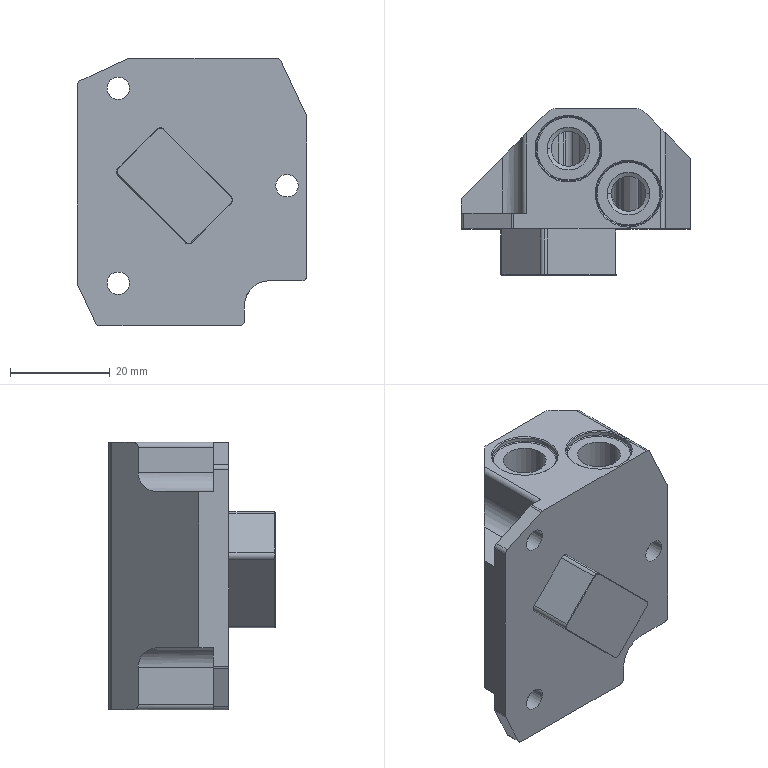NC program | NX | posted with a generic post | part box 46 x 33.25 x 53.5 mm
Whole program, first 1397 of 1693 lines:
N10 G17 G21 G94 G90
(PLANAR_MILL_7 , TOOL : D5-15-D6-50-3T-ROUGH)
N12 T03 M6
N14 G54
N16 G17 G0 G90 X1.887 Y-14.189 B0. C0. S4500 M3
N18 G43 Z20. H3
N20 Z1.
N22 G94 G1 X1.167 Y-14.167 Z0.975 F300.
N24 X0.474 Y-14.445 Z0.949
N26 X-0.055 Y-14.974 Z0.923
N28 X-0.333 Y-15.667 Z0.896
N30 Y-16.333 Z0.873
N32 X-0.055 Y-17.026 Z0.847
N34 X0.474 Y-17.555 Z0.821
N36 X1.167 Y-17.833 Z0.795
N38 X1.833 Z0.772
N40 X2.526 Y-17.555 Z0.746
N42 X3.055 Y-17.026 Z0.719
N44 X3.333 Y-16.333 Z0.693
N46 Y-15.667 Z0.67
N48 X3.055 Y-14.974 Z0.644
N50 X2.526 Y-14.445 Z0.618
N52 X1.833 Y-14.167 Z0.592
N54 X1.167 Z0.569
N56 X0.474 Y-14.445 Z0.542
N58 X-0.055 Y-14.974 Z0.516
N60 X-0.333 Y-15.667 Z0.49
N62 Y-16.333 Z0.467
N64 X-0.055 Y-17.026 Z0.441
N66 X0.474 Y-17.555 Z0.415
N68 X1.167 Y-17.833 Z0.389
N70 X1.833 Z0.366
N72 X2.526 Y-17.555 Z0.339
N74 X3.055 Y-17.026 Z0.313
N76 X3.333 Y-16.333 Z0.287
N78 Y-15.667 Z0.264
N80 X3.055 Y-14.974 Z0.238
N82 X2.526 Y-14.445 Z0.212
N84 X1.833 Y-14.167 Z0.186
N86 X1.167 Z0.162
N88 X0.474 Y-14.445 Z0.136
N90 X-0.055 Y-14.974 Z0.11
N92 X-0.333 Y-15.667 Z0.084
N94 Y-16.333 Z0.061
N96 X-0.055 Y-17.026 Z0.035
N98 X0.474 Y-17.555 Z0.009
N100 X1.167 Y-17.833 Z-0.017
N102 X1.833 Z-0.041
N104 X2.526 Y-17.555 Z-0.067
N106 X3.055 Y-17.026 Z-0.093
N108 X3.333 Y-16.333 Z-0.119
N110 Y-15.667 Z-0.142
N112 X3.055 Y-14.974 Z-0.168
N114 X2.526 Y-14.445 Z-0.194
N116 X1.833 Y-14.167 Z-0.22
N118 X1.167 Z-0.244
N120 X0.474 Y-14.445 Z-0.27
N122 X-0.055 Y-14.974 Z-0.296
N124 X-0.333 Y-15.667 Z-0.322
N126 Y-16.333 Z-0.345
N128 X-0.055 Y-17.026 Z-0.371
N130 X0.474 Y-17.555 Z-0.397
N132 X1.167 Y-17.833 Z-0.423
N134 X1.833 Z-0.447
N136 X2.526 Y-17.555 Z-0.473
N138 X3.055 Y-17.026 Z-0.499
N140 X3.333 Y-16.333 Z-0.525
N142 Y-15.667 Z-0.548
N144 X3.055 Y-14.974 Z-0.574
N146 X2.526 Y-14.445 Z-0.6
N148 X1.833 Y-14.167 Z-0.627
N150 X1.167 Z-0.65
N152 X0.474 Y-14.445 Z-0.676
N154 X-0.055 Y-14.974 Z-0.702
N156 X-0.333 Y-15.667 Z-0.728
N158 Y-16.333 Z-0.751
N160 X-0.055 Y-17.026 Z-0.777
N162 X0.474 Y-17.555 Z-0.804
N164 X1.167 Y-17.833 Z-0.83
N166 X1.833 Z-0.853
N168 X2.526 Y-17.555 Z-0.879
N170 X3.055 Y-17.026 Z-0.905
N172 X3.333 Y-16.333 Z-0.931
N174 Y-15.667 Z-0.954
N176 X3.055 Y-14.974 Z-0.98
N178 X2.526 Y-14.445 Z-1.007
N180 X1.833 Y-14.167 Z-1.033
N182 X1.167 Z-1.056
N184 X0.474 Y-14.445 Z-1.082
N186 X-0.055 Y-14.974 Z-1.108
N188 X-0.333 Y-15.667 Z-1.134
N190 Y-16.333 Z-1.157
N192 X-0.055 Y-17.026 Z-1.184
N194 X0.474 Y-17.555 Z-1.21
N196 X1.167 Y-17.833 Z-1.236
N198 X1.833 Z-1.259
N200 X2.526 Y-17.555 Z-1.285
N202 X3.055 Y-17.026 Z-1.311
N204 X3.333 Y-16.333 Z-1.337
N206 Y-15.667 Z-1.361
N208 X3.055 Y-14.974 Z-1.387
N210 X2.526 Y-14.445 Z-1.413
N212 X1.833 Y-14.167 Z-1.439
N214 X1.167 Z-1.462
N216 X0.474 Y-14.445 Z-1.488
N218 X-0.055 Y-14.974 Z-1.514
N220 X-0.333 Y-15.667 Z-1.54
N222 Y-16.333 Z-1.564
N224 X-0.055 Y-17.026 Z-1.59
N226 X0.474 Y-17.555 Z-1.616
N228 X1.167 Y-17.833 Z-1.642
N230 X1.833 Z-1.665
N232 X2.526 Y-17.555 Z-1.691
N234 X3.055 Y-17.026 Z-1.717
N236 X3.333 Y-16.333 Z-1.743
N238 Y-15.667 Z-1.767
N240 X3.055 Y-14.974 Z-1.793
N242 X2.526 Y-14.445 Z-1.819
N244 X1.833 Y-14.167 Z-1.845
N246 X1.167 Z-1.868
N248 X0.474 Y-14.445 Z-1.894
N250 X-0.055 Y-14.974 Z-1.92
N252 X-0.333 Y-15.667 Z-1.946
N254 Y-16.333 Z-1.97
N256 X-0.055 Y-17.026 Z-1.996
N258 X0.474 Y-17.555 Z-2.022
N260 X1.167 Y-17.833 Z-2.048
N262 X1.833 Z-2.071
N264 X2.526 Y-17.555 Z-2.097
N266 X3.055 Y-17.026 Z-2.123
N268 X3.333 Y-16.333 Z-2.15
N270 Y-15.667 Z-2.173
N272 X3.055 Y-14.974 Z-2.199
N274 X2.526 Y-14.445 Z-2.225
N276 X1.833 Y-14.167 Z-2.251
N278 X1.167 Z-2.274
N280 X0.474 Y-14.445 Z-2.3
N282 X-0.055 Y-14.974 Z-2.326
N284 X-0.333 Y-15.667 Z-2.353
N286 Y-16.333 Z-2.376
N288 X-0.055 Y-17.026 Z-2.402
N290 X0.474 Y-17.555 Z-2.428
N292 X1.167 Y-17.833 Z-2.454
N294 X1.833 Z-2.477
N296 X2.526 Y-17.555 Z-2.503
N298 X3.055 Y-17.026 Z-2.53
N300 X3.333 Y-16.333 Z-2.556
N302 Y-15.667 Z-2.579
N304 X3.055 Y-14.974 Z-2.605
N306 X2.526 Y-14.445 Z-2.631
N308 X1.833 Y-14.167 Z-2.657
N310 X1.167 Z-2.68
N312 X0.474 Y-14.445 Z-2.707
N314 X-0.055 Y-14.974 Z-2.733
N316 X-0.333 Y-15.667 Z-2.759
N318 Y-16.333 Z-2.782
N320 X-0.055 Y-17.026 Z-2.808
N322 X0.474 Y-17.555 Z-2.834
N324 X1.167 Y-17.833 Z-2.86
N326 X1.833 Z-2.884
N328 X2.526 Y-17.555 Z-2.91
N330 X3.055 Y-17.026 Z-2.936
N332 X3.333 Y-16.333 Z-2.962
N334 Y-15.667 Z-2.985
N336 X3.055 Y-14.974 Z-3.011
N338 X2.526 Y-14.445 Z-3.037
N340 X1.833 Y-14.167 Z-3.063
N342 X1.167 Z-3.087
N344 X0.474 Y-14.445 Z-3.113
N346 X-0.055 Y-14.974 Z-3.139
N348 X-0.333 Y-15.667 Z-3.165
N350 Y-16.333 Z-3.188
N352 X-0.055 Y-17.026 Z-3.214
N354 X0.474 Y-17.555 Z-3.24
N356 X1.167 Y-17.833 Z-3.266
N358 X1.833 Z-3.29
N360 X2.526 Y-17.555 Z-3.316
N362 X3.055 Y-17.026 Z-3.342
N364 X3.333 Y-16.333 Z-3.368
N366 Y-15.667 Z-3.391
N368 X3.055 Y-14.974 Z-3.417
N370 X2.526 Y-14.445 Z-3.443
N372 X1.833 Y-14.167 Z-3.469
N374 X1.167 Z-3.493
N376 X0.474 Y-14.445 Z-3.519
N378 X-0.055 Y-14.974 Z-3.545
N380 X-0.333 Y-15.667 Z-3.571
N382 Y-16.333 Z-3.594
N384 X-0.055 Y-17.026 Z-3.62
N386 X0.474 Y-17.555 Z-3.646
N388 X1.167 Y-17.833 Z-3.672
N390 X1.833 Z-3.696
N392 X2.526 Y-17.555 Z-3.722
N394 X3.055 Y-17.026 Z-3.748
N396 X3.333 Y-16.333 Z-3.774
N398 Y-15.667 Z-3.797
N400 X3.055 Y-14.974 Z-3.823
N402 X2.526 Y-14.445 Z-3.849
N404 X1.833 Y-14.167 Z-3.876
N406 X1.167 Z-3.899
N408 X0.474 Y-14.445 Z-3.925
N410 X-0.055 Y-14.974 Z-3.951
N412 X-0.333 Y-15.667 Z-3.977
N414 Y-16.333 Z-4.
N416 X-0.055 Y-17.026 Z-4.026
N418 X0.474 Y-17.555 Z-4.053
N420 X1.167 Y-17.833 Z-4.079
N422 X1.833 Z-4.102
N424 X2.526 Y-17.555 Z-4.128
N426 X3.055 Y-17.026 Z-4.154
N428 X3.333 Y-16.333 Z-4.18
N430 Y-15.667 Z-4.203
N432 X3.055 Y-14.974 Z-4.23
N434 X2.526 Y-14.445 Z-4.256
N436 X1.833 Y-14.167 Z-4.282
N438 X1.167 Z-4.305
N440 X0.474 Y-14.445 Z-4.331
N442 X-0.055 Y-14.974 Z-4.357
N444 X-0.333 Y-15.667 Z-4.383
N446 Y-16.333 Z-4.406
N448 X-0.055 Y-17.026 Z-4.433
N450 X0.474 Y-17.555 Z-4.459
N452 X1.167 Y-17.833 Z-4.485
N454 X1.833 Z-4.508
N456 X2.526 Y-17.555 Z-4.534
N458 X3.055 Y-17.026 Z-4.56
N460 X3.333 Y-16.333 Z-4.586
N462 Y-15.667 Z-4.61
N464 X3.055 Y-14.974 Z-4.636
N466 X2.526 Y-14.445 Z-4.662
N468 X1.833 Y-14.167 Z-4.688
N470 X1.167 Z-4.711
N472 X0.474 Y-14.445 Z-4.737
N474 X-0.055 Y-14.974 Z-4.763
N476 X-0.333 Y-15.667 Z-4.789
N478 Y-16.333 Z-4.813
N480 X-0.055 Y-17.026 Z-4.839
N482 X0.474 Y-17.555 Z-4.865
N484 X1.167 Y-17.833 Z-4.891
N486 X1.833 Z-4.914
N488 X2.526 Y-17.555 Z-4.94
N490 X3.055 Y-17.026 Z-4.966
N492 X3.333 Y-16.333 Z-4.992
N494 Y-15.667 Z-5.016
N496 X3.055 Y-14.974 Z-5.042
N498 X2.526 Y-14.445 Z-5.068
N500 X1.833 Y-14.167 Z-5.094
N502 X1.167 Z-5.117
N504 X0.474 Y-14.445 Z-5.143
N506 X-0.055 Y-14.974 Z-5.169
N508 X-0.333 Y-15.667 Z-5.195
N510 Y-16.333 Z-5.219
N512 X-0.055 Y-17.026 Z-5.245
N514 X0.474 Y-17.555 Z-5.271
N516 X1.167 Y-17.833 Z-5.297
N518 X1.833 Z-5.32
N520 X2.526 Y-17.555 Z-5.346
N522 X3.055 Y-17.026 Z-5.372
N524 X3.333 Y-16.333 Z-5.399
N526 Y-15.667 Z-5.422
N528 X3.055 Y-14.974 Z-5.448
N530 X2.526 Y-14.445 Z-5.474
N532 X1.833 Y-14.167 Z-5.5
N534 X1.167 Z-5.523
N536 X0.474 Y-14.445 Z-5.549
N538 X-0.055 Y-14.974 Z-5.576
N540 X-0.333 Y-15.667 Z-5.602
N542 Y-16.333 Z-5.625
N544 X-0.055 Y-17.026 Z-5.651
N546 X0.474 Y-17.555 Z-5.677
N548 X1.167 Y-17.833 Z-5.703
N550 X1.833 Z-5.726
N552 X2.526 Y-17.555 Z-5.752
N554 X3.055 Y-17.026 Z-5.779
N556 X3.333 Y-16.333 Z-5.805
N558 Y-15.667 Z-5.828
N560 X3.055 Y-14.974 Z-5.854
N562 X2.526 Y-14.445 Z-5.88
N564 X1.833 Y-14.167 Z-5.906
N566 X1.167 Z-5.929
N568 X0.474 Y-14.445 Z-5.956
N570 X-0.055 Y-14.974 Z-5.982
N572 X-0.333 Y-15.667 Z-6.008
N574 Y-16.333 Z-6.031
N576 X-0.055 Y-17.026 Z-6.057
N578 X0.474 Y-17.555 Z-6.083
N580 X1.167 Y-17.833 Z-6.109
N582 X1.833 Z-6.133
N584 X2.526 Y-17.555 Z-6.159
N586 X3.055 Y-17.026 Z-6.185
N588 X3.333 Y-16.333 Z-6.211
N590 Y-15.667 Z-6.234
N592 X3.055 Y-14.974 Z-6.26
N594 X2.526 Y-14.445 Z-6.286
N596 X1.833 Y-14.167 Z-6.312
N598 X1.167 Z-6.336
N600 X0.474 Y-14.445 Z-6.362
N602 X-0.055 Y-14.974 Z-6.388
N604 X-0.333 Y-15.667 Z-6.414
N606 Y-16.333 Z-6.437
N608 X-0.055 Y-17.026 Z-6.463
N610 X0.474 Y-17.555 Z-6.489
N612 X1.167 Y-17.833 Z-6.515
N614 X1.833 Z-6.539
N616 X2.526 Y-17.555 Z-6.565
N618 X3.055 Y-17.026 Z-6.591
N620 X3.333 Y-16.333 Z-6.617
N622 Y-15.667 Z-6.64
N624 X3.055 Y-14.974 Z-6.666
N626 X2.526 Y-14.445 Z-6.692
N628 X1.833 Y-14.167 Z-6.718
N630 X1.167 Z-6.742
N632 X0.474 Y-14.445 Z-6.768
N634 X-0.055 Y-14.974 Z-6.794
N636 X-0.333 Y-15.667 Z-6.82
N638 Y-16.333 Z-6.843
N640 X-0.055 Y-17.026 Z-6.869
N642 X0.474 Y-17.555 Z-6.895
N644 X1.167 Y-17.833 Z-6.922
N646 X1.833 Z-6.945
N648 X2.526 Y-17.555 Z-6.971
N650 X3.055 Y-17.026 Z-6.997
N652 X3.333 Y-16.333 Z-7.023
N654 Y-15.667 Z-7.046
N656 X3.055 Y-14.974 Z-7.072
N658 X2.526 Y-14.445 Z-7.098
N660 X1.833 Y-14.167 Z-7.125
N662 X1.167 Z-7.148
N664 X0.474 Y-14.445 Z-7.174
N666 X-0.055 Y-14.974 Z-7.2
N668 X-0.333 Y-15.667 Z-7.226
N670 Y-16.333 Z-7.249
N672 X-0.055 Y-17.026 Z-7.275
N674 X0.474 Y-17.555 Z-7.302
N676 X1.167 Y-17.833 Z-7.328
N678 X1.833 Z-7.351
N680 X2.526 Y-17.555 Z-7.377
N682 X3.055 Y-17.026 Z-7.403
N684 X3.333 Y-16.333 Z-7.429
N686 Y-15.667 Z-7.452
N688 X3.055 Y-14.974 Z-7.479
N690 X2.526 Y-14.445 Z-7.505
N692 X1.833 Y-14.167 Z-7.531
N694 X1.167 Z-7.554
N696 X0.474 Y-14.445 Z-7.58
N698 X-0.055 Y-14.974 Z-7.606
N700 X-0.333 Y-15.667 Z-7.632
N702 Y-16.333 Z-7.656
N704 X-0.055 Y-17.026 Z-7.682
N706 X0.474 Y-17.555 Z-7.708
N708 X1.167 Y-17.833 Z-7.734
N710 X1.833 Z-7.757
N712 X2.526 Y-17.555 Z-7.783
N714 X3.055 Y-17.026 Z-7.809
N716 X3.333 Y-16.333 Z-7.835
N718 Y-15.667 Z-7.859
N720 X3.055 Y-14.974 Z-7.885
N722 X2.526 Y-14.445 Z-7.911
N724 X1.833 Y-14.167 Z-7.937
N726 X1.167 Z-7.96
N728 X0.474 Y-14.445 Z-7.986
N730 X-0.055 Y-14.974 Z-8.012
N732 X-0.333 Y-15.667 Z-8.038
N734 Y-16. Z-8.05
N736 G3 X1.5 Y-17.833 R1.833
N738 X-0.333 Y-16. R-1.833
N740 G1 Z-7.05
N742 G0 Z20.
N744 X-10.113 Y-5.189
N746 Z1.
N748 G1 X-10.833 Y-5.167 Z0.975
N750 X-11.526 Y-5.445 Z0.949
N752 X-12.055 Y-5.974 Z0.923
N754 X-12.333 Y-6.667 Z0.896
N756 Y-7.333 Z0.873
N758 X-12.055 Y-8.026 Z0.847
N760 X-11.526 Y-8.555 Z0.821
N762 X-10.833 Y-8.833 Z0.795
N764 X-10.167 Z0.772
N766 X-9.474 Y-8.555 Z0.746
N768 X-8.945 Y-8.026 Z0.719
N770 X-8.667 Y-7.333 Z0.693
N772 Y-6.667 Z0.67
N774 X-8.945 Y-5.974 Z0.644
N776 X-9.474 Y-5.445 Z0.618
N778 X-10.167 Y-5.167 Z0.592
N780 X-10.833 Z0.569
N782 X-11.526 Y-5.445 Z0.542
N784 X-12.055 Y-5.974 Z0.516
N786 X-12.333 Y-6.667 Z0.49
N788 Y-7.333 Z0.467
N790 X-12.055 Y-8.026 Z0.441
N792 X-11.526 Y-8.555 Z0.415
N794 X-10.833 Y-8.833 Z0.389
N796 X-10.167 Z0.366
N798 X-9.474 Y-8.555 Z0.339
N800 X-8.945 Y-8.026 Z0.313
N802 X-8.667 Y-7.333 Z0.287
N804 Y-6.667 Z0.264
N806 X-8.945 Y-5.974 Z0.238
N808 X-9.474 Y-5.445 Z0.212
N810 X-10.167 Y-5.167 Z0.186
N812 X-10.833 Z0.162
N814 X-11.526 Y-5.445 Z0.136
N816 X-12.055 Y-5.974 Z0.11
N818 X-12.333 Y-6.667 Z0.084
N820 Y-7.333 Z0.061
N822 X-12.055 Y-8.026 Z0.035
N824 X-11.526 Y-8.555 Z0.009
N826 X-10.833 Y-8.833 Z-0.017
N828 X-10.167 Z-0.041
N830 X-9.474 Y-8.555 Z-0.067
N832 X-8.945 Y-8.026 Z-0.093
N834 X-8.667 Y-7.333 Z-0.119
N836 Y-6.667 Z-0.142
N838 X-8.945 Y-5.974 Z-0.168
N840 X-9.474 Y-5.445 Z-0.194
N842 X-10.167 Y-5.167 Z-0.22
N844 X-10.833 Z-0.244
N846 X-11.526 Y-5.445 Z-0.27
N848 X-12.055 Y-5.974 Z-0.296
N850 X-12.333 Y-6.667 Z-0.322
N852 Y-7.333 Z-0.345
N854 X-12.055 Y-8.026 Z-0.371
N856 X-11.526 Y-8.555 Z-0.397
N858 X-10.833 Y-8.833 Z-0.423
N860 X-10.167 Z-0.447
N862 X-9.474 Y-8.555 Z-0.473
N864 X-8.945 Y-8.026 Z-0.499
N866 X-8.667 Y-7.333 Z-0.525
N868 Y-6.667 Z-0.548
N870 X-8.945 Y-5.974 Z-0.574
N872 X-9.474 Y-5.445 Z-0.6
N874 X-10.167 Y-5.167 Z-0.627
N876 X-10.833 Z-0.65
N878 X-11.526 Y-5.445 Z-0.676
N880 X-12.055 Y-5.974 Z-0.702
N882 X-12.333 Y-6.667 Z-0.728
N884 Y-7.333 Z-0.751
N886 X-12.055 Y-8.026 Z-0.777
N888 X-11.526 Y-8.555 Z-0.804
N890 X-10.833 Y-8.833 Z-0.83
N892 X-10.167 Z-0.853
N894 X-9.474 Y-8.555 Z-0.879
N896 X-8.945 Y-8.026 Z-0.905
N898 X-8.667 Y-7.333 Z-0.931
N900 Y-6.667 Z-0.954
N902 X-8.945 Y-5.974 Z-0.98
N904 X-9.474 Y-5.445 Z-1.007
N906 X-10.167 Y-5.167 Z-1.033
N908 X-10.833 Z-1.056
N910 X-11.526 Y-5.445 Z-1.082
N912 X-12.055 Y-5.974 Z-1.108
N914 X-12.333 Y-6.667 Z-1.134
N916 Y-7.333 Z-1.157
N918 X-12.055 Y-8.026 Z-1.184
N920 X-11.526 Y-8.555 Z-1.21
N922 X-10.833 Y-8.833 Z-1.236
N924 X-10.167 Z-1.259
N926 X-9.474 Y-8.555 Z-1.285
N928 X-8.945 Y-8.026 Z-1.311
N930 X-8.667 Y-7.333 Z-1.337
N932 Y-6.667 Z-1.361
N934 X-8.945 Y-5.974 Z-1.387
N936 X-9.474 Y-5.445 Z-1.413
N938 X-10.167 Y-5.167 Z-1.439
N940 X-10.833 Z-1.462
N942 X-11.526 Y-5.445 Z-1.488
N944 X-12.055 Y-5.974 Z-1.514
N946 X-12.333 Y-6.667 Z-1.54
N948 Y-7.333 Z-1.564
N950 X-12.055 Y-8.026 Z-1.59
N952 X-11.526 Y-8.555 Z-1.616
N954 X-10.833 Y-8.833 Z-1.642
N956 X-10.167 Z-1.665
N958 X-9.474 Y-8.555 Z-1.691
N960 X-8.945 Y-8.026 Z-1.717
N962 X-8.667 Y-7.333 Z-1.743
N964 Y-6.667 Z-1.767
N966 X-8.945 Y-5.974 Z-1.793
N968 X-9.474 Y-5.445 Z-1.819
N970 X-10.167 Y-5.167 Z-1.845
N972 X-10.833 Z-1.868
N974 X-11.526 Y-5.445 Z-1.894
N976 X-12.055 Y-5.974 Z-1.92
N978 X-12.333 Y-6.667 Z-1.946
N980 Y-7.333 Z-1.97
N982 X-12.055 Y-8.026 Z-1.996
N984 X-11.526 Y-8.555 Z-2.022
N986 X-10.833 Y-8.833 Z-2.048
N988 X-10.167 Z-2.071
N990 X-9.474 Y-8.555 Z-2.097
N992 X-8.945 Y-8.026 Z-2.123
N994 X-8.667 Y-7.333 Z-2.15
N996 Y-6.667 Z-2.173
N998 X-8.945 Y-5.974 Z-2.199
N1000 X-9.474 Y-5.445 Z-2.225
N1002 X-10.167 Y-5.167 Z-2.251
N1004 X-10.833 Z-2.274
N1006 X-11.526 Y-5.445 Z-2.3
N1008 X-12.055 Y-5.974 Z-2.326
N1010 X-12.333 Y-6.667 Z-2.353
N1012 Y-7.333 Z-2.376
N1014 X-12.055 Y-8.026 Z-2.402
N1016 X-11.526 Y-8.555 Z-2.428
N1018 X-10.833 Y-8.833 Z-2.454
N1020 X-10.167 Z-2.477
N1022 X-9.474 Y-8.555 Z-2.503
N1024 X-8.945 Y-8.026 Z-2.53
N1026 X-8.667 Y-7.333 Z-2.556
N1028 Y-6.667 Z-2.579
N1030 X-8.945 Y-5.974 Z-2.605
N1032 X-9.474 Y-5.445 Z-2.631
N1034 X-10.167 Y-5.167 Z-2.657
N1036 X-10.833 Z-2.68
N1038 X-11.526 Y-5.445 Z-2.707
N1040 X-12.055 Y-5.974 Z-2.733
N1042 X-12.333 Y-6.667 Z-2.759
N1044 Y-7.333 Z-2.782
N1046 X-12.055 Y-8.026 Z-2.808
N1048 X-11.526 Y-8.555 Z-2.834
N1050 X-10.833 Y-8.833 Z-2.86
N1052 X-10.167 Z-2.884
N1054 X-9.474 Y-8.555 Z-2.91
N1056 X-8.945 Y-8.026 Z-2.936
N1058 X-8.667 Y-7.333 Z-2.962
N1060 Y-6.667 Z-2.985
N1062 X-8.945 Y-5.974 Z-3.011
N1064 X-9.474 Y-5.445 Z-3.037
N1066 X-10.167 Y-5.167 Z-3.063
N1068 X-10.833 Z-3.087
N1070 X-11.526 Y-5.445 Z-3.113
N1072 X-12.055 Y-5.974 Z-3.139
N1074 X-12.333 Y-6.667 Z-3.165
N1076 Y-7.333 Z-3.188
N1078 X-12.055 Y-8.026 Z-3.214
N1080 X-11.526 Y-8.555 Z-3.24
N1082 X-10.833 Y-8.833 Z-3.266
N1084 X-10.167 Z-3.29
N1086 X-9.474 Y-8.555 Z-3.316
N1088 X-8.945 Y-8.026 Z-3.342
N1090 X-8.667 Y-7.333 Z-3.368
N1092 Y-6.667 Z-3.391
N1094 X-8.945 Y-5.974 Z-3.417
N1096 X-9.474 Y-5.445 Z-3.443
N1098 X-10.167 Y-5.167 Z-3.469
N1100 X-10.833 Z-3.493
N1102 X-11.526 Y-5.445 Z-3.519
N1104 X-12.055 Y-5.974 Z-3.545
N1106 X-12.333 Y-6.667 Z-3.571
N1108 Y-7.333 Z-3.594
N1110 X-12.055 Y-8.026 Z-3.62
N1112 X-11.526 Y-8.555 Z-3.646
N1114 X-10.833 Y-8.833 Z-3.672
N1116 X-10.167 Z-3.696
N1118 X-9.474 Y-8.555 Z-3.722
N1120 X-8.945 Y-8.026 Z-3.748
N1122 X-8.667 Y-7.333 Z-3.774
N1124 Y-6.667 Z-3.797
N1126 X-8.945 Y-5.974 Z-3.823
N1128 X-9.474 Y-5.445 Z-3.849
N1130 X-10.167 Y-5.167 Z-3.876
N1132 X-10.833 Z-3.899
N1134 X-11.526 Y-5.445 Z-3.925
N1136 X-12.055 Y-5.974 Z-3.951
N1138 X-12.333 Y-6.667 Z-3.977
N1140 Y-7.333 Z-4.
N1142 X-12.055 Y-8.026 Z-4.026
N1144 X-11.526 Y-8.555 Z-4.053
N1146 X-10.833 Y-8.833 Z-4.079
N1148 X-10.167 Z-4.102
N1150 X-9.474 Y-8.555 Z-4.128
N1152 X-8.945 Y-8.026 Z-4.154
N1154 X-8.667 Y-7.333 Z-4.18
N1156 Y-6.667 Z-4.203
N1158 X-8.945 Y-5.974 Z-4.23
N1160 X-9.474 Y-5.445 Z-4.256
N1162 X-10.167 Y-5.167 Z-4.282
N1164 X-10.833 Z-4.305
N1166 X-11.526 Y-5.445 Z-4.331
N1168 X-12.055 Y-5.974 Z-4.357
N1170 X-12.333 Y-6.667 Z-4.383
N1172 Y-7.333 Z-4.406
N1174 X-12.055 Y-8.026 Z-4.433
N1176 X-11.526 Y-8.555 Z-4.459
N1178 X-10.833 Y-8.833 Z-4.485
N1180 X-10.167 Z-4.508
N1182 X-9.474 Y-8.555 Z-4.534
N1184 X-8.945 Y-8.026 Z-4.56
N1186 X-8.667 Y-7.333 Z-4.586
N1188 Y-6.667 Z-4.61
N1190 X-8.945 Y-5.974 Z-4.636
N1192 X-9.474 Y-5.445 Z-4.662
N1194 X-10.167 Y-5.167 Z-4.688
N1196 X-10.833 Z-4.711
N1198 X-11.526 Y-5.445 Z-4.737
N1200 X-12.055 Y-5.974 Z-4.763
N1202 X-12.333 Y-6.667 Z-4.789
N1204 Y-7.333 Z-4.813
N1206 X-12.055 Y-8.026 Z-4.839
N1208 X-11.526 Y-8.555 Z-4.865
N1210 X-10.833 Y-8.833 Z-4.891
N1212 X-10.167 Z-4.914
N1214 X-9.474 Y-8.555 Z-4.94
N1216 X-8.945 Y-8.026 Z-4.966
N1218 X-8.667 Y-7.333 Z-4.992
N1220 Y-6.667 Z-5.016
N1222 X-8.945 Y-5.974 Z-5.042
N1224 X-9.474 Y-5.445 Z-5.068
N1226 X-10.167 Y-5.167 Z-5.094
N1228 X-10.833 Z-5.117
N1230 X-11.526 Y-5.445 Z-5.143
N1232 X-12.055 Y-5.974 Z-5.169
N1234 X-12.333 Y-6.667 Z-5.195
N1236 Y-7.333 Z-5.219
N1238 X-12.055 Y-8.026 Z-5.245
N1240 X-11.526 Y-8.555 Z-5.271
N1242 X-10.833 Y-8.833 Z-5.297
N1244 X-10.167 Z-5.32
N1246 X-9.474 Y-8.555 Z-5.346
N1248 X-8.945 Y-8.026 Z-5.372
N1250 X-8.667 Y-7.333 Z-5.399
N1252 Y-6.667 Z-5.422
N1254 X-8.945 Y-5.974 Z-5.448
N1256 X-9.474 Y-5.445 Z-5.474
N1258 X-10.167 Y-5.167 Z-5.5
N1260 X-10.833 Z-5.523
N1262 X-11.526 Y-5.445 Z-5.549
N1264 X-12.055 Y-5.974 Z-5.576
N1266 X-12.333 Y-6.667 Z-5.602
N1268 Y-7.333 Z-5.625
N1270 X-12.055 Y-8.026 Z-5.651
N1272 X-11.526 Y-8.555 Z-5.677
N1274 X-10.833 Y-8.833 Z-5.703
N1276 X-10.167 Z-5.726
N1278 X-9.474 Y-8.555 Z-5.752
N1280 X-8.945 Y-8.026 Z-5.779
N1282 X-8.667 Y-7.333 Z-5.805
N1284 Y-6.667 Z-5.828
N1286 X-8.945 Y-5.974 Z-5.854
N1288 X-9.474 Y-5.445 Z-5.88
N1290 X-10.167 Y-5.167 Z-5.906
N1292 X-10.833 Z-5.929
N1294 X-11.526 Y-5.445 Z-5.956
N1296 X-12.055 Y-5.974 Z-5.982
N1298 X-12.333 Y-6.667 Z-6.008
N1300 Y-7.333 Z-6.031
N1302 X-12.055 Y-8.026 Z-6.057
N1304 X-11.526 Y-8.555 Z-6.083
N1306 X-10.833 Y-8.833 Z-6.109
N1308 X-10.167 Z-6.133
N1310 X-9.474 Y-8.555 Z-6.159
N1312 X-8.945 Y-8.026 Z-6.185
N1314 X-8.667 Y-7.333 Z-6.211
N1316 Y-6.667 Z-6.234
N1318 X-8.945 Y-5.974 Z-6.26
N1320 X-9.474 Y-5.445 Z-6.286
N1322 X-10.167 Y-5.167 Z-6.312
N1324 X-10.833 Z-6.336
N1326 X-11.526 Y-5.445 Z-6.362
N1328 X-12.055 Y-5.974 Z-6.388
N1330 X-12.333 Y-6.667 Z-6.414
N1332 Y-7.333 Z-6.437
N1334 X-12.055 Y-8.026 Z-6.463
N1336 X-11.526 Y-8.555 Z-6.489
N1338 X-10.833 Y-8.833 Z-6.515
N1340 X-10.167 Z-6.539
N1342 X-9.474 Y-8.555 Z-6.565
N1344 X-8.945 Y-8.026 Z-6.591
N1346 X-8.667 Y-7.333 Z-6.617
N1348 Y-6.667 Z-6.64
N1350 X-8.945 Y-5.974 Z-6.666
N1352 X-9.474 Y-5.445 Z-6.692
N1354 X-10.167 Y-5.167 Z-6.718
N1356 X-10.833 Z-6.742
N1358 X-11.526 Y-5.445 Z-6.768
N1360 X-12.055 Y-5.974 Z-6.794
N1362 X-12.333 Y-6.667 Z-6.82
N1364 Y-7.333 Z-6.843
N1366 X-12.055 Y-8.026 Z-6.869
N1368 X-11.526 Y-8.555 Z-6.895
N1370 X-10.833 Y-8.833 Z-6.922
N1372 X-10.167 Z-6.945
N1374 X-9.474 Y-8.555 Z-6.971
N1376 X-8.945 Y-8.026 Z-6.997
N1378 X-8.667 Y-7.333 Z-7.023
N1380 Y-6.667 Z-7.046
N1382 X-8.945 Y-5.974 Z-7.072
N1384 X-9.474 Y-5.445 Z-7.098
N1386 X-10.167 Y-5.167 Z-7.125
N1388 X-10.833 Z-7.148
N1390 X-11.526 Y-5.445 Z-7.174
N1392 X-12.055 Y-5.974 Z-7.2
N1394 X-12.333 Y-6.667 Z-7.226
N1396 Y-7.333 Z-7.249
N1398 X-12.055 Y-8.026 Z-7.275
N1400 X-11.526 Y-8.555 Z-7.302
N1402 X-10.833 Y-8.833 Z-7.328
N1404 X-10.167 Z-7.351
N1406 X-9.474 Y-8.555 Z-7.377
N1408 X-8.945 Y-8.026 Z-7.403
N1410 X-8.667 Y-7.333 Z-7.429
N1412 Y-6.667 Z-7.452
N1414 X-8.945 Y-5.974 Z-7.479
N1416 X-9.474 Y-5.445 Z-7.505
N1418 X-10.167 Y-5.167 Z-7.531
N1420 X-10.833 Z-7.554
N1422 X-11.526 Y-5.445 Z-7.58
N1424 X-12.055 Y-5.974 Z-7.606
N1426 X-12.333 Y-6.667 Z-7.632
N1428 Y-7.333 Z-7.656
N1430 X-12.055 Y-8.026 Z-7.682
N1432 X-11.526 Y-8.555 Z-7.708
N1434 X-10.833 Y-8.833 Z-7.734
N1436 X-10.167 Z-7.757
N1438 X-9.474 Y-8.555 Z-7.783
N1440 X-8.945 Y-8.026 Z-7.809
N1442 X-8.667 Y-7.333 Z-7.835
N1444 Y-6.667 Z-7.859
N1446 X-8.945 Y-5.974 Z-7.885
N1448 X-9.474 Y-5.445 Z-7.911
N1450 X-10.167 Y-5.167 Z-7.937
N1452 X-10.833 Z-7.96
N1454 X-11.526 Y-5.445 Z-7.986
N1456 X-12.055 Y-5.974 Z-8.012
N1458 X-12.333 Y-6.667 Z-8.038
N1460 Y-7. Z-8.05
N1462 G3 X-10.5 Y-8.833 R1.833
N1464 X-12.333 Y-7. R-1.833
N1466 G1 Z-7.05
N1468 G0 Z20.
(PLANAR_MILL_7_COPY_1 , TOOL : D5-15-D6-50-3T-ROUGH)
N1470 X-10.995 Y-6.14
N1472 Z-7.5
N1474 G1 X-11.228 Y-6.272 Z-7.509
N1476 X-11.5 Y-6.753 Z-7.529
N1478 Y-7.247 Z-7.546
N1480 X-11.228 Y-7.728 Z-7.565
N1482 X-10.747 Y-8. Z-7.585
N1484 X-10.253 Z-7.602
N1486 X-9.772 Y-7.728 Z-7.621
N1488 X-9.5 Y-7.247 Z-7.64
N1490 Y-6.753 Z-7.658
N1492 X-9.772 Y-6.272 Z-7.677
N1494 X-10.253 Y-6. Z-7.696
N1496 X-10.747 Z-7.713
N1498 X-11.228 Y-6.272 Z-7.733
N1500 X-11.5 Y-6.753 Z-7.752
N1502 Y-7.247 Z-7.769
N1504 X-11.228 Y-7.728 Z-7.789
N1506 X-10.747 Y-8. Z-7.808
N1508 X-10.253 Z-7.825
N1510 X-9.772 Y-7.728 Z-7.844
N1512 X-9.5 Y-7.247 Z-7.864
N1514 Y-6.753 Z-7.881
N1516 X-9.772 Y-6.272 Z-7.9
N1518 X-10.253 Y-6. Z-7.92
N1520 X-10.747 Z-7.937
N1522 X-11.228 Y-6.272 Z-7.956
N1524 X-11.5 Y-6.753 Z-7.975
N1526 Y-7.247 Z-7.993
N1528 X-11.228 Y-7.728 Z-8.012
N1530 X-10.747 Y-8. Z-8.031
N1532 X-10.253 Z-8.049
N1534 X-9.772 Y-7.728 Z-8.068
N1536 X-9.5 Y-7.247 Z-8.087
N1538 Y-6.753 Z-8.104
N1540 X-9.772 Y-6.272 Z-8.124
N1542 X-10.253 Y-6. Z-8.143
N1544 X-10.747 Z-8.16
N1546 X-11.228 Y-6.272 Z-8.18
N1548 X-11.5 Y-6.753 Z-8.199
N1550 Y-7.247 Z-8.216
N1552 X-11.228 Y-7.728 Z-8.235
N1554 X-10.747 Y-8. Z-8.255
N1556 X-10.253 Z-8.272
N1558 X-9.772 Y-7.728 Z-8.291
N1560 X-9.5 Y-7.247 Z-8.311
N1562 Y-6.753 Z-8.328
N1564 X-9.772 Y-6.272 Z-8.347
N1566 X-10.253 Y-6. Z-8.366
N1568 X-10.747 Z-8.384
N1570 X-11.228 Y-6.272 Z-8.403
N1572 X-11.5 Y-6.753 Z-8.422
N1574 Y-7.247 Z-8.44
N1576 X-11.228 Y-7.728 Z-8.459
N1578 X-10.747 Y-8. Z-8.478
N1580 X-10.253 Z-8.495
N1582 X-9.772 Y-7.728 Z-8.515
N1584 X-9.5 Y-7.247 Z-8.534
N1586 Y-6.753 Z-8.551
N1588 X-9.772 Y-6.272 Z-8.571
N1590 X-10.253 Y-6. Z-8.59
N1592 X-10.747 Z-8.607
N1594 X-11.228 Y-6.272 Z-8.626
N1596 X-11.5 Y-6.753 Z-8.646
N1598 Y-7.247 Z-8.663
N1600 X-11.228 Y-7.728 Z-8.682
N1602 X-10.747 Y-8. Z-8.702
N1604 X-10.253 Z-8.719
N1606 X-9.772 Y-7.728 Z-8.738
N1608 X-9.5 Y-7.247 Z-8.757
N1610 Y-6.753 Z-8.775
N1612 X-9.772 Y-6.272 Z-8.794
N1614 X-10.253 Y-6. Z-8.813
N1616 X-10.747 Z-8.83
N1618 X-11.228 Y-6.272 Z-8.85
N1620 X-11.5 Y-6.753 Z-8.869
N1622 Y-7.247 Z-8.886
N1624 X-11.228 Y-7.728 Z-8.906
N1626 X-10.747 Y-8. Z-8.925
N1628 X-10.253 Z-8.942
N1630 X-9.772 Y-7.728 Z-8.961
N1632 X-9.5 Y-7.247 Z-8.981
N1634 Y-6.753 Z-8.998
N1636 X-9.772 Y-6.272 Z-9.017
N1638 X-10.253 Y-6. Z-9.037
N1640 X-10.747 Z-9.054
N1642 X-11.228 Y-6.272 Z-9.073
N1644 X-11.5 Y-6.753 Z-9.092
N1646 Y-7.247 Z-9.11
N1648 X-11.228 Y-7.728 Z-9.129
N1650 X-10.747 Y-8. Z-9.148
N1652 X-10.253 Z-9.166
N1654 X-9.772 Y-7.728 Z-9.185
N1656 X-9.5 Y-7.247 Z-9.204
N1658 Y-6.753 Z-9.221
N1660 X-9.772 Y-6.272 Z-9.241
N1662 X-10.253 Y-6. Z-9.26
N1664 X-10.747 Z-9.277
N1666 X-11.228 Y-6.272 Z-9.297
N1668 X-11.5 Y-6.753 Z-9.316
N1670 Y-7.247 Z-9.333
N1672 X-11.228 Y-7.728 Z-9.352
N1674 X-10.747 Y-8. Z-9.372
N1676 X-10.253 Z-9.389
N1678 X-9.772 Y-7.728 Z-9.408
N1680 X-9.5 Y-7.247 Z-9.428
N1682 Y-6.753 Z-9.445
N1684 X-9.772 Y-6.272 Z-9.464
N1686 X-10.253 Y-6. Z-9.483
N1688 X-10.747 Z-9.501
N1690 X-11.228 Y-6.272 Z-9.52
N1692 X-11.5 Y-6.753 Z-9.539
N1694 Y-7.247 Z-9.557
N1696 X-11.228 Y-7.728 Z-9.576
N1698 X-10.747 Y-8. Z-9.595
N1700 X-10.253 Z-9.612
N1702 X-9.772 Y-7.728 Z-9.632
N1704 X-9.5 Y-7.247 Z-9.651
N1706 Y-6.753 Z-9.668
N1708 X-9.772 Y-6.272 Z-9.688
N1710 X-10.253 Y-6. Z-9.707
N1712 X-10.747 Z-9.724
N1714 X-11.228 Y-6.272 Z-9.743
N1716 X-11.5 Y-6.753 Z-9.763
N1718 Y-7.247 Z-9.78
N1720 X-11.228 Y-7.728 Z-9.799
N1722 X-10.747 Y-8. Z-9.819
N1724 X-10.253 Z-9.836
N1726 X-9.772 Y-7.728 Z-9.855
N1728 X-9.5 Y-7.247 Z-9.874
N1730 Y-6.753 Z-9.892
N1732 X-9.772 Y-6.272 Z-9.911
N1734 X-10.253 Y-6. Z-9.93
N1736 X-10.747 Z-9.947
N1738 X-11.228 Y-6.272 Z-9.967
N1740 X-11.5 Y-6.753 Z-9.986
N1742 Y-7.247 Z-10.003
N1744 X-11.228 Y-7.728 Z-10.023
N1746 X-10.747 Y-8. Z-10.042
N1748 X-10.253 Z-10.059
N1750 X-9.772 Y-7.728 Z-10.078
N1752 X-9.5 Y-7.247 Z-10.098
N1754 Y-6.753 Z-10.115
N1756 X-9.772 Y-6.272 Z-10.134
N1758 X-10.253 Y-6. Z-10.154
N1760 X-10.747 Z-10.171
N1762 X-11.228 Y-6.272 Z-10.19
N1764 X-11.5 Y-6.753 Z-10.209
N1766 Y-7.247 Z-10.227
N1768 X-11.228 Y-7.728 Z-10.246
N1770 X-10.747 Y-8. Z-10.265
N1772 X-10.253 Z-10.283
N1774 X-9.772 Y-7.728 Z-10.302
N1776 X-9.5 Y-7.247 Z-10.321
N1778 Y-6.753 Z-10.338
N1780 X-9.772 Y-6.272 Z-10.358
N1782 X-10.253 Y-6. Z-10.377
N1784 X-10.747 Z-10.394
N1786 X-11.228 Y-6.272 Z-10.414
N1788 X-11.5 Y-6.753 Z-10.433
N1790 Y-7.247 Z-10.45
N1792 X-11.228 Y-7.728 Z-10.469
N1794 X-10.747 Y-8. Z-10.489
N1796 X-10.253 Z-10.506
N1798 X-9.772 Y-7.728 Z-10.525
N1800 X-9.5 Y-7.247 Z-10.545
N1802 Y-6.753 Z-10.562
N1804 X-9.772 Y-6.272 Z-10.581
N1806 X-10.253 Y-6. Z-10.6
N1808 X-10.747 Z-10.618
N1810 X-11.228 Y-6.272 Z-10.637
N1812 X-11.5 Y-6.753 Z-10.656
N1814 Y-7.247 Z-10.674
N1816 X-11.228 Y-7.728 Z-10.693
N1818 X-10.747 Y-8. Z-10.712
N1820 X-10.253 Z-10.729
N1822 X-9.772 Y-7.728 Z-10.749
N1824 X-9.5 Y-7.247 Z-10.768
N1826 Y-6.753 Z-10.785
N1828 X-9.772 Y-6.272 Z-10.805
N1830 X-10.253 Y-6. Z-10.824
N1832 X-10.747 Z-10.841
N1834 X-11.228 Y-6.272 Z-10.86
N1836 X-11.5 Y-6.753 Z-10.88
N1838 Y-7.247 Z-10.897
N1840 X-11.228 Y-7.728 Z-10.916
N1842 X-10.747 Y-8. Z-10.936
N1844 X-10.253 Z-10.953
N1846 X-9.772 Y-7.728 Z-10.972
N1848 X-9.5 Y-7.247 Z-10.991
N1850 Y-7. Z-11.
N1852 G3 X-10.5 Y-6. R1.
N1854 X-9.5 Y-7. R-1.
N1856 G1 Z-10.
N1858 G0 Z20.
N1860 X1.005 Y-15.14
N1862 Z-7.5
N1864 G1 X0.772 Y-15.272 Z-7.509
N1866 X0.5 Y-15.753 Z-7.529
N1868 Y-16.247 Z-7.546
N1870 X0.772 Y-16.728 Z-7.565
N1872 X1.253 Y-17. Z-7.585
N1874 X1.747 Z-7.602
N1876 X2.228 Y-16.728 Z-7.621
N1878 X2.5 Y-16.247 Z-7.64
N1880 Y-15.753 Z-7.658
N1882 X2.228 Y-15.272 Z-7.677
N1884 X1.747 Y-15. Z-7.696
N1886 X1.253 Z-7.713
N1888 X0.772 Y-15.272 Z-7.733
N1890 X0.5 Y-15.753 Z-7.752
N1892 Y-16.247 Z-7.769
N1894 X0.772 Y-16.728 Z-7.789
N1896 X1.253 Y-17. Z-7.808
N1898 X1.747 Z-7.825
N1900 X2.228 Y-16.728 Z-7.844
N1902 X2.5 Y-16.247 Z-7.864
N1904 Y-15.753 Z-7.881
N1906 X2.228 Y-15.272 Z-7.9
N1908 X1.747 Y-15. Z-7.92
N1910 X1.253 Z-7.937
N1912 X0.772 Y-15.272 Z-7.956
N1914 X0.5 Y-15.753 Z-7.975
N1916 Y-16.247 Z-7.993
N1918 X0.772 Y-16.728 Z-8.012
N1920 X1.253 Y-17. Z-8.031
N1922 X1.747 Z-8.049
N1924 X2.228 Y-16.728 Z-8.068
N1926 X2.5 Y-16.247 Z-8.087
N1928 Y-15.753 Z-8.104
N1930 X2.228 Y-15.272 Z-8.124
N1932 X1.747 Y-15. Z-8.143
N1934 X1.253 Z-8.16
N1936 X0.772 Y-15.272 Z-8.18
N1938 X0.5 Y-15.753 Z-8.199
N1940 Y-16.247 Z-8.216
N1942 X0.772 Y-16.728 Z-8.235
N1944 X1.253 Y-17. Z-8.255
N1946 X1.747 Z-8.272
N1948 X2.228 Y-16.728 Z-8.291
N1950 X2.5 Y-16.247 Z-8.311
N1952 Y-15.753 Z-8.328
N1954 X2.228 Y-15.272 Z-8.347
N1956 X1.747 Y-15. Z-8.366
N1958 X1.253 Z-8.384
N1960 X0.772 Y-15.272 Z-8.403
N1962 X0.5 Y-15.753 Z-8.422
N1964 Y-16.247 Z-8.44
N1966 X0.772 Y-16.728 Z-8.459
N1968 X1.253 Y-17. Z-8.478
N1970 X1.747 Z-8.495
N1972 X2.228 Y-16.728 Z-8.515
N1974 X2.5 Y-16.247 Z-8.534
N1976 Y-15.753 Z-8.551
N1978 X2.228 Y-15.272 Z-8.571
N1980 X1.747 Y-15. Z-8.59
N1982 X1.253 Z-8.607
N1984 X0.772 Y-15.272 Z-8.626
N1986 X0.5 Y-15.753 Z-8.646
N1988 Y-16.247 Z-8.663
N1990 X0.772 Y-16.728 Z-8.682
N1992 X1.253 Y-17. Z-8.702
N1994 X1.747 Z-8.719
N1996 X2.228 Y-16.728 Z-8.738
N1998 X2.5 Y-16.247 Z-8.757
N2000 Y-15.753 Z-8.775
N2002 X2.228 Y-15.272 Z-8.794
N2004 X1.747 Y-15. Z-8.813
N2006 X1.253 Z-8.83
N2008 X0.772 Y-15.272 Z-8.85
N2010 X0.5 Y-15.753 Z-8.869
N2012 Y-16.247 Z-8.886
N2014 X0.772 Y-16.728 Z-8.906
N2016 X1.253 Y-17. Z-8.925
N2018 X1.747 Z-8.942
N2020 X2.228 Y-16.728 Z-8.961
N2022 X2.5 Y-16.247 Z-8.981
N2024 Y-15.753 Z-8.998
N2026 X2.228 Y-15.272 Z-9.017
N2028 X1.747 Y-15. Z-9.037
N2030 X1.253 Z-9.054
N2032 X0.772 Y-15.272 Z-9.073
N2034 X0.5 Y-15.753 Z-9.092
N2036 Y-16.247 Z-9.11
N2038 X0.772 Y-16.728 Z-9.129
N2040 X1.253 Y-17. Z-9.148
N2042 X1.747 Z-9.166
N2044 X2.228 Y-16.728 Z-9.185
N2046 X2.5 Y-16.247 Z-9.204
N2048 Y-15.753 Z-9.221
N2050 X2.228 Y-15.272 Z-9.241
N2052 X1.747 Y-15. Z-9.26
N2054 X1.253 Z-9.277
N2056 X0.772 Y-15.272 Z-9.297
N2058 X0.5 Y-15.753 Z-9.316
N2060 Y-16.247 Z-9.333
N2062 X0.772 Y-16.728 Z-9.352
N2064 X1.253 Y-17. Z-9.372
N2066 X1.747 Z-9.389
N2068 X2.228 Y-16.728 Z-9.408
N2070 X2.5 Y-16.247 Z-9.428
N2072 Y-15.753 Z-9.445
N2074 X2.228 Y-15.272 Z-9.464
N2076 X1.747 Y-15. Z-9.483
N2078 X1.253 Z-9.501
N2080 X0.772 Y-15.272 Z-9.52
N2082 X0.5 Y-15.753 Z-9.539
N2084 Y-16.247 Z-9.557
N2086 X0.772 Y-16.728 Z-9.576
N2088 X1.253 Y-17. Z-9.595
N2090 X1.747 Z-9.612
N2092 X2.228 Y-16.728 Z-9.632
N2094 X2.5 Y-16.247 Z-9.651
N2096 Y-15.753 Z-9.668
N2098 X2.228 Y-15.272 Z-9.688
N2100 X1.747 Y-15. Z-9.707
N2102 X1.253 Z-9.724
N2104 X0.772 Y-15.272 Z-9.743
N2106 X0.5 Y-15.753 Z-9.763
N2108 Y-16.247 Z-9.78
N2110 X0.772 Y-16.728 Z-9.799
N2112 X1.253 Y-17. Z-9.819
N2114 X1.747 Z-9.836
N2116 X2.228 Y-16.728 Z-9.855
N2118 X2.5 Y-16.247 Z-9.874
N2120 Y-15.753 Z-9.892
N2122 X2.228 Y-15.272 Z-9.911
N2124 X1.747 Y-15. Z-9.93
N2126 X1.253 Z-9.947
N2128 X0.772 Y-15.272 Z-9.967
N2130 X0.5 Y-15.753 Z-9.986
N2132 Y-16.247 Z-10.003
N2134 X0.772 Y-16.728 Z-10.023
N2136 X1.253 Y-17. Z-10.042
N2138 X1.747 Z-10.059
N2140 X2.228 Y-16.728 Z-10.078
N2142 X2.5 Y-16.247 Z-10.098
N2144 Y-15.753 Z-10.115
N2146 X2.228 Y-15.272 Z-10.134
N2148 X1.747 Y-15. Z-10.154
N2150 X1.253 Z-10.171
N2152 X0.772 Y-15.272 Z-10.19
N2154 X0.5 Y-15.753 Z-10.209
N2156 Y-16.247 Z-10.227
N2158 X0.772 Y-16.728 Z-10.246
N2160 X1.253 Y-17. Z-10.265
N2162 X1.747 Z-10.283
N2164 X2.228 Y-16.728 Z-10.302
N2166 X2.5 Y-16.247 Z-10.321
N2168 Y-15.753 Z-10.338
N2170 X2.228 Y-15.272 Z-10.358
N2172 X1.747 Y-15. Z-10.377
N2174 X1.253 Z-10.394
N2176 X0.772 Y-15.272 Z-10.414
N2178 X0.5 Y-15.753 Z-10.433
N2180 Y-16.247 Z-10.45
N2182 X0.772 Y-16.728 Z-10.469
N2184 X1.253 Y-17. Z-10.489
N2186 X1.747 Z-10.506
N2188 X2.228 Y-16.728 Z-10.525
N2190 X2.5 Y-16.247 Z-10.545
N2192 Y-15.753 Z-10.562
N2194 X2.228 Y-15.272 Z-10.581
N2196 X1.747 Y-15. Z-10.6
N2198 X1.253 Z-10.618
N2200 X0.772 Y-15.272 Z-10.637
N2202 X0.5 Y-15.753 Z-10.656
N2204 Y-16.247 Z-10.674
N2206 X0.772 Y-16.728 Z-10.693
N2208 X1.253 Y-17. Z-10.712
N2210 X1.747 Z-10.729
N2212 X2.228 Y-16.728 Z-10.749
N2214 X2.5 Y-16.247 Z-10.768
N2216 Y-15.753 Z-10.785
N2218 X2.228 Y-15.272 Z-10.805
N2220 X1.747 Y-15. Z-10.824
N2222 X1.253 Z-10.841
N2224 X0.772 Y-15.272 Z-10.86
N2226 X0.5 Y-15.753 Z-10.88
N2228 Y-16.247 Z-10.897
N2230 X0.772 Y-16.728 Z-10.916
N2232 X1.253 Y-17. Z-10.936
N2234 X1.747 Z-10.953
N2236 X2.228 Y-16.728 Z-10.972
N2238 X2.5 Y-16.247 Z-10.991
N2240 Y-16. Z-11.
N2242 G3 X1.5 Y-15. R1.
N2244 X2.5 Y-16. R-1.
N2246 G1 Z-10.
N2248 G0 Z20.
N2250 M5
(PLANAR_MILL_4 , TOOL : D3R0.2)
N2252 T10 M6
N2254 G54
N2256 G17 G0 G90 X-11.643 Y-2.199 B0. C0. S4500 M3
N2258 G43 Z20. H10
N2260 Z1.
N2262 G94 G1 X-12.347 Y-2.375 Z0.994 F600.
N2264 X-13.515 Y-3.036 Z0.982
N2266 X-14.464 Y-3.985 Z0.97
N2268 X-15.125 Y-5.153 Z0.959
N2270 X-15.45 Y-6.454 Z0.947
N2272 Y-7.546 Z0.937
N2274 X-15.125 Y-8.847 Z0.926
N2276 X-14.464 Y-10.015 Z0.914
N2278 X-13.515 Y-10.964 Z0.902
N2280 X-12.347 Y-11.625 Z0.89
N2282 X-11.046 Y-11.95 Z0.879
N2284 X-9.954 Z0.869
N2286 X-8.653 Y-11.625 Z0.858
N2288 X-7.485 Y-10.964 Z0.846
N2290 X-6.536 Y-10.015 Z0.834
N2292 X-5.875 Y-8.847 Z0.822
N2294 X-5.55 Y-7.546 Z0.811
N2296 Y-6.454 Z0.801
N2298 X-5.875 Y-5.153 Z0.789
N2300 X-6.536 Y-3.985 Z0.778
N2302 X-7.485 Y-3.036 Z0.766
N2304 X-8.653 Y-2.375 Z0.754
N2306 X-9.954 Y-2.05 Z0.743
N2308 X-11.046 Z0.733
N2310 X-12.347 Y-2.375 Z0.721
N2312 X-13.515 Y-3.036 Z0.71
N2314 X-14.464 Y-3.985 Z0.698
N2316 X-15.125 Y-5.153 Z0.686
N2318 X-15.45 Y-6.454 Z0.675
N2320 Y-7.546 Z0.665
N2322 X-15.125 Y-8.847 Z0.653
N2324 X-14.464 Y-10.015 Z0.642
N2326 X-13.515 Y-10.964 Z0.63
N2328 X-12.347 Y-11.625 Z0.618
N2330 X-11.046 Y-11.95 Z0.606
N2332 X-9.954 Z0.597
N2334 X-8.653 Y-11.625 Z0.585
N2336 X-7.485 Y-10.964 Z0.574
N2338 X-6.536 Y-10.015 Z0.562
N2340 X-5.875 Y-8.847 Z0.55
N2342 X-5.55 Y-7.546 Z0.538
N2344 Y-6.454 Z0.529
N2346 X-5.875 Y-5.153 Z0.517
N2348 X-6.536 Y-3.985 Z0.505
N2350 X-7.485 Y-3.036 Z0.494
N2352 X-8.653 Y-2.375 Z0.482
N2354 X-9.954 Y-2.05 Z0.47
N2356 X-11.046 Z0.461
N2358 X-12.347 Y-2.375 Z0.449
N2360 X-13.515 Y-3.036 Z0.437
N2362 X-14.464 Y-3.985 Z0.426
N2364 X-15.125 Y-5.153 Z0.414
N2366 X-15.45 Y-6.454 Z0.402
N2368 Y-7.546 Z0.393
N2370 X-15.125 Y-8.847 Z0.381
N2372 X-14.464 Y-10.015 Z0.369
N2374 X-13.515 Y-10.964 Z0.358
N2376 X-12.347 Y-11.625 Z0.346
N2378 X-11.046 Y-11.95 Z0.334
N2380 X-9.954 Z0.325
N2382 X-8.653 Y-11.625 Z0.313
N2384 X-7.485 Y-10.964 Z0.301
N2386 X-6.536 Y-10.015 Z0.29
N2388 X-5.875 Y-8.847 Z0.278
N2390 X-5.55 Y-7.546 Z0.266
N2392 Y-6.454 Z0.257
N2394 X-5.875 Y-5.153 Z0.245
N2396 X-6.536 Y-3.985 Z0.233
N2398 X-7.485 Y-3.036 Z0.221
N2400 X-8.653 Y-2.375 Z0.21
N2402 X-9.954 Y-2.05 Z0.198
N2404 X-11.046 Z0.189
N2406 X-12.347 Y-2.375 Z0.177
N2408 X-13.515 Y-3.036 Z0.165
N2410 X-14.464 Y-3.985 Z0.153
N2412 X-15.125 Y-5.153 Z0.142
N2414 X-15.45 Y-6.454 Z0.13
N2416 Y-7.546 Z0.12
N2418 X-15.125 Y-8.847 Z0.109
N2420 X-14.464 Y-10.015 Z0.097
N2422 X-13.515 Y-10.964 Z0.085
N2424 X-12.347 Y-11.625 Z0.074
N2426 X-11.046 Y-11.95 Z0.062
N2428 X-9.954 Z0.052
N2430 X-8.653 Y-11.625 Z0.041
N2432 X-7.485 Y-10.964 Z0.029
N2434 X-6.536 Y-10.015 Z0.017
N2436 X-5.875 Y-8.847 Z0.006
N2438 X-5.55 Y-7.546 Z-0.006
N2440 Y-6.454 Z-0.016
N2442 X-5.875 Y-5.153 Z-0.027
N2444 X-6.536 Y-3.985 Z-0.039
N2446 X-7.485 Y-3.036 Z-0.051
N2448 X-8.653 Y-2.375 Z-0.062
N2450 X-9.954 Y-2.05 Z-0.074
N2452 X-11.046 Z-0.084
N2454 X-12.347 Y-2.375 Z-0.095
N2456 X-13.515 Y-3.036 Z-0.107
N2458 X-14.464 Y-3.985 Z-0.119
N2460 X-15.125 Y-5.153 Z-0.131
N2462 X-15.45 Y-6.454 Z-0.142
N2464 Y-7.546 Z-0.152
N2466 X-15.125 Y-8.847 Z-0.164
N2468 X-14.464 Y-10.015 Z-0.175
N2470 X-13.515 Y-10.964 Z-0.187
N2472 X-12.347 Y-11.625 Z-0.199
N2474 X-11.046 Y-11.95 Z-0.21
N2476 X-9.954 Z-0.22
N2478 X-8.653 Y-11.625 Z-0.232
N2480 X-7.485 Y-10.964 Z-0.243
N2482 X-6.536 Y-10.015 Z-0.255
N2484 X-5.875 Y-8.847 Z-0.267
N2486 X-5.55 Y-7.546 Z-0.278
N2488 Y-6.454 Z-0.288
N2490 X-5.875 Y-5.153 Z-0.3
N2492 X-6.536 Y-3.985 Z-0.311
N2494 X-7.485 Y-3.036 Z-0.323
N2496 X-8.653 Y-2.375 Z-0.335
N2498 X-9.954 Y-2.05 Z-0.346
N2500 X-11.046 Z-0.356
N2502 X-12.347 Y-2.375 Z-0.368
N2504 X-13.515 Y-3.036 Z-0.379
N2506 X-14.464 Y-3.985 Z-0.391
N2508 X-15.125 Y-5.153 Z-0.403
N2510 X-15.45 Y-6.454 Z-0.415
N2512 Y-7.546 Z-0.424
N2514 X-15.125 Y-8.847 Z-0.436
N2516 X-14.464 Y-10.015 Z-0.447
N2518 X-13.515 Y-10.964 Z-0.459
N2520 X-12.347 Y-11.625 Z-0.471
N2522 X-11.046 Y-11.95 Z-0.483
N2524 X-9.954 Z-0.492
N2526 X-8.653 Y-11.625 Z-0.504
N2528 X-7.485 Y-10.964 Z-0.516
N2530 X-6.536 Y-10.015 Z-0.527
N2532 X-5.875 Y-8.847 Z-0.539
N2534 X-5.55 Y-7.546 Z-0.551
N2536 Y-6.454 Z-0.56
N2538 X-5.875 Y-5.153 Z-0.572
N2540 X-6.536 Y-3.985 Z-0.584
N2542 X-7.485 Y-3.036 Z-0.595
N2544 X-8.653 Y-2.375 Z-0.607
N2546 X-9.954 Y-2.05 Z-0.619
N2548 X-11.046 Z-0.628
N2550 X-12.347 Y-2.375 Z-0.64
N2552 X-13.515 Y-3.036 Z-0.652
N2554 X-14.464 Y-3.985 Z-0.663
N2556 X-15.125 Y-5.153 Z-0.675
N2558 X-15.45 Y-6.454 Z-0.687
N2560 Y-7.546 Z-0.696
N2562 X-15.125 Y-8.847 Z-0.708
N2564 X-14.464 Y-10.015 Z-0.72
N2566 X-13.515 Y-10.964 Z-0.731
N2568 X-12.347 Y-11.625 Z-0.743
N2570 X-11.046 Y-11.95 Z-0.755
N2572 X-9.954 Z-0.764
N2574 X-8.653 Y-11.625 Z-0.776
N2576 X-7.485 Y-10.964 Z-0.788
N2578 X-6.536 Y-10.015 Z-0.8
N2580 X-5.875 Y-8.847 Z-0.811
N2582 X-5.55 Y-7.546 Z-0.823
N2584 Y-6.454 Z-0.832
N2586 X-5.875 Y-5.153 Z-0.844
N2588 X-6.536 Y-3.985 Z-0.856
N2590 X-7.485 Y-3.036 Z-0.868
N2592 X-8.653 Y-2.375 Z-0.879
N2594 X-9.954 Y-2.05 Z-0.891
N2596 X-11.046 Z-0.901
N2598 X-12.347 Y-2.375 Z-0.912
N2600 X-13.515 Y-3.036 Z-0.924
N2602 X-14.464 Y-3.985 Z-0.936
N2604 X-15.125 Y-5.153 Z-0.947
N2606 X-15.45 Y-6.454 Z-0.959
N2608 Y-7.546 Z-0.969
N2610 X-15.125 Y-8.847 Z-0.98
N2612 X-14.464 Y-10.015 Z-0.992
N2614 X-13.515 Y-10.964 Z-1.004
N2616 X-12.347 Y-11.625 Z-1.015
N2618 X-11.046 Y-11.95 Z-1.027
N2620 X-9.954 Z-1.037
N2622 X-8.653 Y-11.625 Z-1.048
N2624 X-7.485 Y-10.964 Z-1.06
N2626 X-6.536 Y-10.015 Z-1.072
N2628 X-5.875 Y-8.847 Z-1.084
N2630 X-5.55 Y-7.546 Z-1.095
N2632 Y-7. Z-1.1
N2634 G3 X-10.5 Y-2.05 R4.95
N2636 X-5.55 Y-7. R-4.95
N2638 G1 Z-0.1
N2640 G0 Z20.
N2642 X0.357 Y-11.199
N2644 Z1.
N2646 G1 X-0.347 Y-11.375 Z0.994
N2648 X-1.515 Y-12.036 Z0.982
N2650 X-2.464 Y-12.985 Z0.97
N2652 X-3.125 Y-14.153 Z0.959
N2654 X-3.45 Y-15.454 Z0.947
N2656 Y-16.546 Z0.937
N2658 X-3.125 Y-17.847 Z0.926
N2660 X-2.464 Y-19.015 Z0.914
N2662 X-1.515 Y-19.964 Z0.902
N2664 X-0.347 Y-20.625 Z0.89
N2666 X0.954 Y-20.95 Z0.879
N2668 X2.046 Z0.869
N2670 X3.347 Y-20.625 Z0.858
N2672 X4.515 Y-19.964 Z0.846
N2674 X5.464 Y-19.015 Z0.834
N2676 X6.125 Y-17.847 Z0.822
N2678 X6.45 Y-16.546 Z0.811
N2680 Y-15.454 Z0.801
N2682 X6.125 Y-14.153 Z0.789
N2684 X5.464 Y-12.985 Z0.778
N2686 X4.515 Y-12.036 Z0.766
N2688 X3.347 Y-11.375 Z0.754
N2690 X2.046 Y-11.05 Z0.743
N2692 X0.954 Z0.733
N2694 X-0.347 Y-11.375 Z0.721
N2696 X-1.515 Y-12.036 Z0.71
N2698 X-2.464 Y-12.985 Z0.698
N2700 X-3.125 Y-14.153 Z0.686
N2702 X-3.45 Y-15.454 Z0.675
N2704 Y-16.546 Z0.665
N2706 X-3.125 Y-17.847 Z0.653
N2708 X-2.464 Y-19.015 Z0.642
N2710 X-1.515 Y-19.964 Z0.63
N2712 X-0.347 Y-20.625 Z0.618
N2714 X0.954 Y-20.95 Z0.606
N2716 X2.046 Z0.597
N2718 X3.347 Y-20.625 Z0.585
N2720 X4.515 Y-19.964 Z0.574
N2722 X5.464 Y-19.015 Z0.562
N2724 X6.125 Y-17.847 Z0.55
N2726 X6.45 Y-16.546 Z0.538
N2728 Y-15.454 Z0.529
N2730 X6.125 Y-14.153 Z0.517
N2732 X5.464 Y-12.985 Z0.505
N2734 X4.515 Y-12.036 Z0.494
N2736 X3.347 Y-11.375 Z0.482
N2738 X2.046 Y-11.05 Z0.47
N2740 X0.954 Z0.461
N2742 X-0.347 Y-11.375 Z0.449
N2744 X-1.515 Y-12.036 Z0.437
N2746 X-2.464 Y-12.985 Z0.426
N2748 X-3.125 Y-14.153 Z0.414
N2750 X-3.45 Y-15.454 Z0.402
N2752 Y-16.546 Z0.393
N2754 X-3.125 Y-17.847 Z0.381
N2756 X-2.464 Y-19.015 Z0.369
N2758 X-1.515 Y-19.964 Z0.358
N2760 X-0.347 Y-20.625 Z0.346
N2762 X0.954 Y-20.95 Z0.334
N2764 X2.046 Z0.325
N2766 X3.347 Y-20.625 Z0.313
N2768 X4.515 Y-19.964 Z0.301
N2770 X5.464 Y-19.015 Z0.29
N2772 X6.125 Y-17.847 Z0.278
N2774 X6.45 Y-16.546 Z0.266
N2776 Y-15.454 Z0.257
N2778 X6.125 Y-14.153 Z0.245
N2780 X5.464 Y-12.985 Z0.233
N2782 X4.515 Y-12.036 Z0.221
N2784 X3.347 Y-11.375 Z0.21
N2786 X2.046 Y-11.05 Z0.198
N2788 X0.954 Z0.189
N2790 X-0.347 Y-11.375 Z0.177
N2792 X-1.515 Y-12.036 Z0.165
N2794 X-2.464 Y-12.985 Z0.153
N2796 X-3.125 Y-14.153 Z0.142